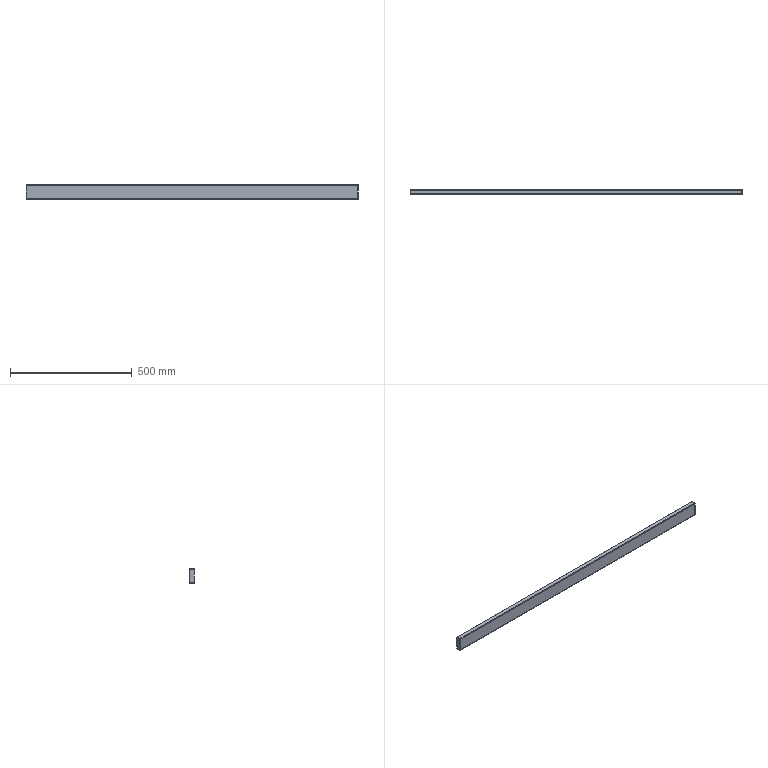Part | SolidWorks | features FlatPattern 5, EdgeFlange 2, SMBaseFlange 2, SheetMetal 2, HoleWzd 1, ICE 1, LPattern 1, MirrorSolid 1 | 7 solids | 90 faces | box 1364 x 20 x 60 mm | volume 253951 mm3 | plane 66 | cylinder 24 | commonest cylinder face diameters 7 x12 5 x8 4 x4